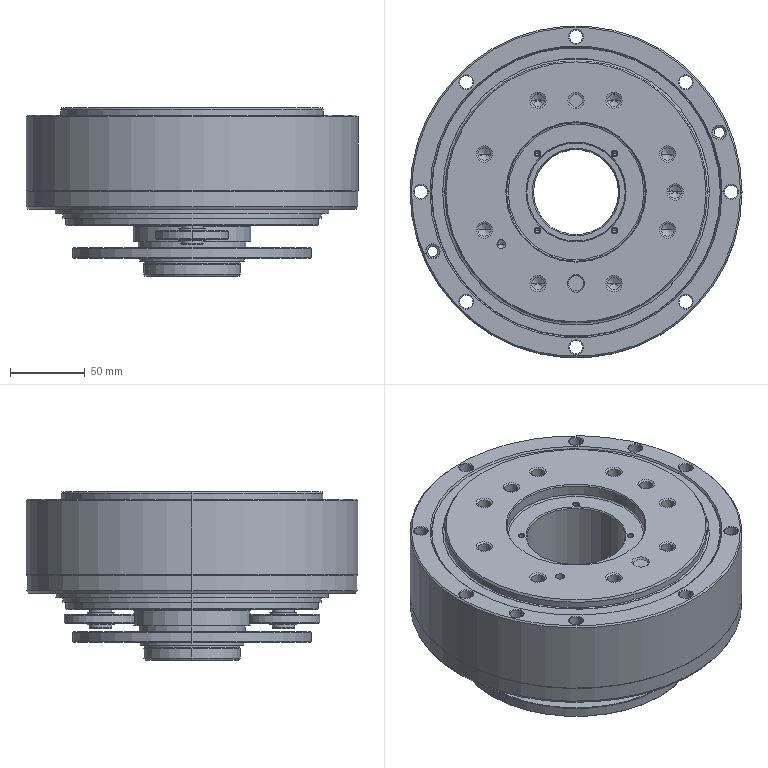Part | 1 solid | 446 faces | box 222.5 x 222.5 x 113 mm | volume 2646292 mm3 | cone 188 | cylinder 156 | plane 90 | torus 12 | commonest cylinder face diameters 9 x20 8.5 x18 13 x12 14 x12 3.3 x8 15 x8